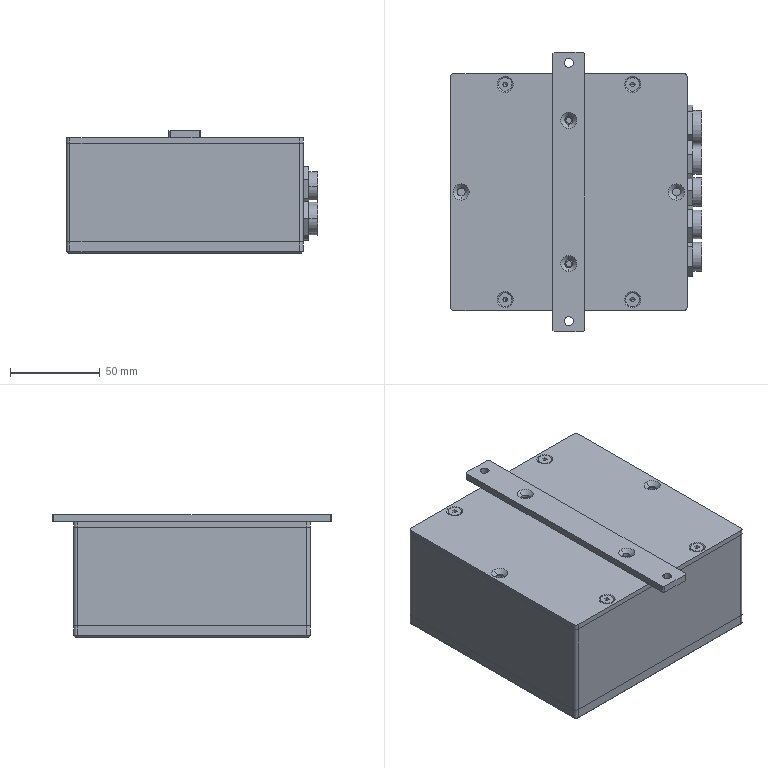Part | STEP file | WG310-Xcont roller(new cable outlet)^Take-up web-guide assembly | 12 solids | 1836 faces | box 140 x 156 x 68.5 mm | volume 333647 mm3 | plane 1119 | cylinder 541 | spline 102 | cone 64 | torus 8 | sphere 2 | commonest cylinder face diameters 2.5 x127 4 x72 2 x47 4.5 x39 6 x28 10 x26